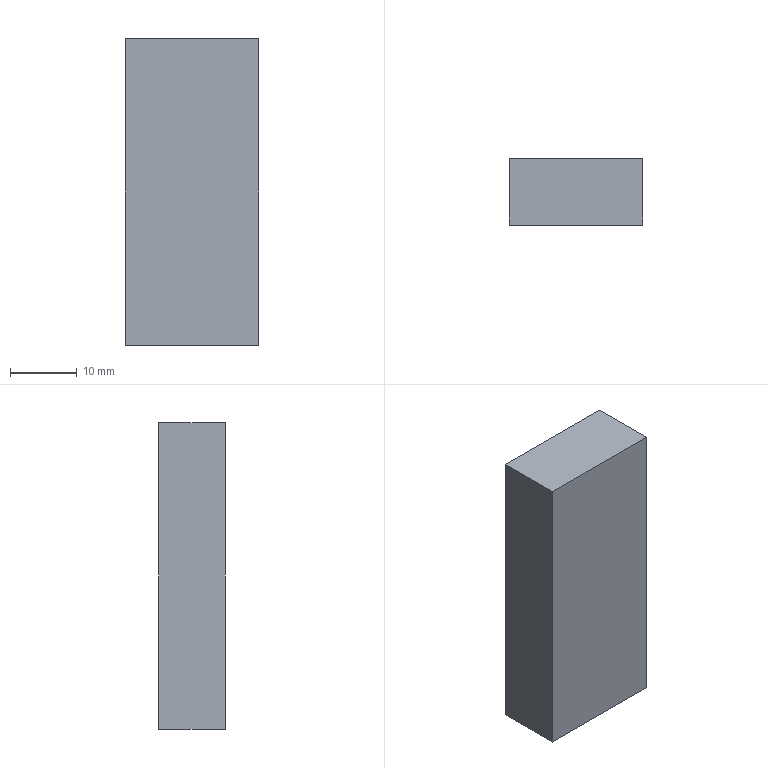Part | NX | features solid 2 | 1 solid | 6 faces | box 20 x 10 x 46 mm | volume 9200 mm3 | plane 6
STEP:
#1=CARTESIAN_POINT('',(-65.,417.,-27.));
#2=VERTEX_POINT('',#1);
#3=CARTESIAN_POINT('',(-65.,427.,-27.));
#4=VERTEX_POINT('',#3);
#5=CARTESIAN_POINT('',(-65.,417.,-27.));
#6=DIRECTION('',(0.,1.,0.));
#7=VECTOR('',#6,1000.);
#8=LINE('',#5,#7);
#9=EDGE_CURVE('',#2,#4,#8,.T.);
#10=ORIENTED_EDGE('',*,*,#9,.T.);
#11=CARTESIAN_POINT('',(-85.,427.,-27.));
#12=VERTEX_POINT('',#11);
#13=CARTESIAN_POINT('',(-85.,427.,-27.));
#14=DIRECTION('',(1.,0.,0.));
#15=VECTOR('',#14,1000.);
#16=LINE('',#13,#15);
#17=EDGE_CURVE('',#12,#4,#16,.T.);
#18=ORIENTED_EDGE('',*,*,#17,.F.);
#19=CARTESIAN_POINT('',(-85.,417.,-27.));
#20=VERTEX_POINT('',#19);
#21=CARTESIAN_POINT('',(-85.,417.,-27.));
#22=DIRECTION('',(0.,-1.,0.));
#23=VECTOR('',#22,1000.);
#24=LINE('',#21,#23);
#25=EDGE_CURVE('',#20,#12,#24,.F.);
#26=ORIENTED_EDGE('',*,*,#25,.F.);
#27=CARTESIAN_POINT('',(-85.,417.,-27.));
#28=DIRECTION('',(1.,0.,0.));
#29=VECTOR('',#28,1000.);
#30=LINE('',#27,#29);
#31=EDGE_CURVE('',#20,#2,#30,.T.);
#32=ORIENTED_EDGE('',*,*,#31,.T.);
#33=EDGE_LOOP('',(#10,#18,#26,#32));
#34=FACE_BOUND('',#33,.T.);
#35=CARTESIAN_POINT('',(-85.,417.,-27.));
#36=DIRECTION('',(0.,0.,1.));
#37=DIRECTION('',(1.,0.,0.));
#38=AXIS2_PLACEMENT_3D('',#35,#36,#37);
#39=PLANE('',#38);
#40=ADVANCED_FACE('',(#34),#39,.T.);
#41=ORIENTED_EDGE('',*,*,#25,.T.);
#42=CARTESIAN_POINT('',(-85.,427.,-73.));
#43=VERTEX_POINT('',#42);
#44=CARTESIAN_POINT('',(-85.,427.,27.));
#45=DIRECTION('',(0.,0.,-1.));
#46=VECTOR('',#45,1000.);
#47=LINE('',#44,#46);
#48=EDGE_CURVE('',#12,#43,#47,.T.);
#49=ORIENTED_EDGE('',*,*,#48,.T.);
#50=CARTESIAN_POINT('',(-85.,417.,-73.));
#51=VERTEX_POINT('',#50);
#52=CARTESIAN_POINT('',(-85.,417.,-73.));
#53=DIRECTION('',(0.,1.,0.));
#54=VECTOR('',#53,1000.);
#55=LINE('',#52,#54);
#56=EDGE_CURVE('',#51,#43,#55,.T.);
#57=ORIENTED_EDGE('',*,*,#56,.F.);
#58=CARTESIAN_POINT('',(-85.,417.,27.));
#59=DIRECTION('',(0.,0.,-1.));
#60=VECTOR('',#59,1000.);
#61=LINE('',#58,#60);
#62=EDGE_CURVE('',#20,#51,#61,.T.);
#63=ORIENTED_EDGE('',*,*,#62,.F.);
#64=EDGE_LOOP('',(#41,#49,#57,#63));
#65=FACE_BOUND('',#64,.T.);
#66=CARTESIAN_POINT('',(-85.,417.,27.));
#67=DIRECTION('',(1.,0.,0.));
#68=DIRECTION('',(0.,0.,-1.));
#69=AXIS2_PLACEMENT_3D('',#66,#67,#68);
#70=PLANE('',#69);
#71=ADVANCED_FACE('',(#65),#70,.F.);
#72=ORIENTED_EDGE('',*,*,#56,.T.);
#73=CARTESIAN_POINT('',(-65.,427.,-73.));
#74=VERTEX_POINT('',#73);
#75=CARTESIAN_POINT('',(-85.,427.,-73.));
#76=DIRECTION('',(-1.,0.,0.));
#77=VECTOR('',#76,1000.);
#78=LINE('',#75,#77);
#79=EDGE_CURVE('',#43,#74,#78,.F.);
#80=ORIENTED_EDGE('',*,*,#79,.T.);
#81=CARTESIAN_POINT('',(-65.,417.,-73.));
#82=VERTEX_POINT('',#81);
#83=CARTESIAN_POINT('',(-65.,417.,-73.));
#84=DIRECTION('',(0.,1.,0.));
#85=VECTOR('',#84,1000.);
#86=LINE('',#83,#85);
#87=EDGE_CURVE('',#82,#74,#86,.T.);
#88=ORIENTED_EDGE('',*,*,#87,.F.);
#89=CARTESIAN_POINT('',(-85.,417.,-73.));
#90=DIRECTION('',(1.,0.,0.));
#91=VECTOR('',#90,1000.);
#92=LINE('',#89,#91);
#93=EDGE_CURVE('',#51,#82,#92,.T.);
#94=ORIENTED_EDGE('',*,*,#93,.F.);
#95=EDGE_LOOP('',(#72,#80,#88,#94));
#96=FACE_BOUND('',#95,.T.);
#97=CARTESIAN_POINT('',(-85.,417.,-73.));
#98=DIRECTION('',(0.,0.,1.));
#99=DIRECTION('',(1.,0.,0.));
#100=AXIS2_PLACEMENT_3D('',#97,#98,#99);
#101=PLANE('',#100);
#102=ADVANCED_FACE('',(#96),#101,.F.);
#103=CARTESIAN_POINT('',(-65.,417.,27.));
#104=DIRECTION('',(0.,0.,-1.));
#105=VECTOR('',#104,1000.);
#106=LINE('',#103,#105);
#107=EDGE_CURVE('',#2,#82,#106,.T.);
#108=ORIENTED_EDGE('',*,*,#107,.T.);
#109=ORIENTED_EDGE('',*,*,#87,.T.);
#110=CARTESIAN_POINT('',(-65.,427.,27.));
#111=DIRECTION('',(0.,0.,-1.));
#112=VECTOR('',#111,1000.);
#113=LINE('',#110,#112);
#114=EDGE_CURVE('',#4,#74,#113,.T.);
#115=ORIENTED_EDGE('',*,*,#114,.F.);
#116=ORIENTED_EDGE('',*,*,#9,.F.);
#117=EDGE_LOOP('',(#108,#109,#115,#116));
#118=FACE_BOUND('',#117,.T.);
#119=CARTESIAN_POINT('',(-65.,417.,27.));
#120=DIRECTION('',(1.,0.,0.));
#121=DIRECTION('',(0.,0.,-1.));
#122=AXIS2_PLACEMENT_3D('',#119,#120,#121);
#123=PLANE('',#122);
#124=ADVANCED_FACE('',(#118),#123,.T.);
#125=ORIENTED_EDGE('',*,*,#79,.F.);
#126=ORIENTED_EDGE('',*,*,#48,.F.);
#127=ORIENTED_EDGE('',*,*,#17,.T.);
#128=ORIENTED_EDGE('',*,*,#114,.T.);
#129=EDGE_LOOP('',(#125,#126,#127,#128));
#130=FACE_BOUND('',#129,.T.);
#131=CARTESIAN_POINT('',(-85.,427.,27.));
#132=DIRECTION('',(0.,-1.,0.));
#133=DIRECTION('',(0.,0.,-1.));
#134=AXIS2_PLACEMENT_3D('',#131,#132,#133);
#135=PLANE('',#134);
#136=ADVANCED_FACE('',(#130),#135,.F.);
#137=ORIENTED_EDGE('',*,*,#93,.T.);
#138=ORIENTED_EDGE('',*,*,#107,.F.);
#139=ORIENTED_EDGE('',*,*,#31,.F.);
#140=ORIENTED_EDGE('',*,*,#62,.T.);
#141=EDGE_LOOP('',(#137,#138,#139,#140));
#142=FACE_BOUND('',#141,.T.);
#143=CARTESIAN_POINT('',(-85.,417.,27.));
#144=DIRECTION('',(0.,-1.,0.));
#145=DIRECTION('',(0.,0.,-1.));
#146=AXIS2_PLACEMENT_3D('',#143,#144,#145);
#147=PLANE('',#146);
#148=ADVANCED_FACE('',(#142),#147,.T.);
#149=CLOSED_SHELL('',(#40,#71,#102,#124,#136,#148));
#150=MANIFOLD_SOLID_BREP('',#149);
#151=(LENGTH_UNIT()NAMED_UNIT(*)SI_UNIT(.MILLI.,.METRE.));
#152=UNCERTAINTY_MEASURE_WITH_UNIT(LENGTH_MEASURE(0.00001),#151,'','');
#153=(NAMED_UNIT(*)PLANE_ANGLE_UNIT()SI_UNIT($,.RADIAN.));
#154=(NAMED_UNIT(*)SI_UNIT($,.STERADIAN.)SOLID_ANGLE_UNIT());
#155=(GEOMETRIC_REPRESENTATION_CONTEXT(3)GLOBAL_UNCERTAINTY_ASSIGNED_CONTEXT((#152))GLOBAL_UNIT_ASSIGNED_CONTEXT((#151,#153,#154))REPRESENTATION_CONTEXT('',''));
#156=ADVANCED_BREP_SHAPE_REPRESENTATION('',(#150),#155);